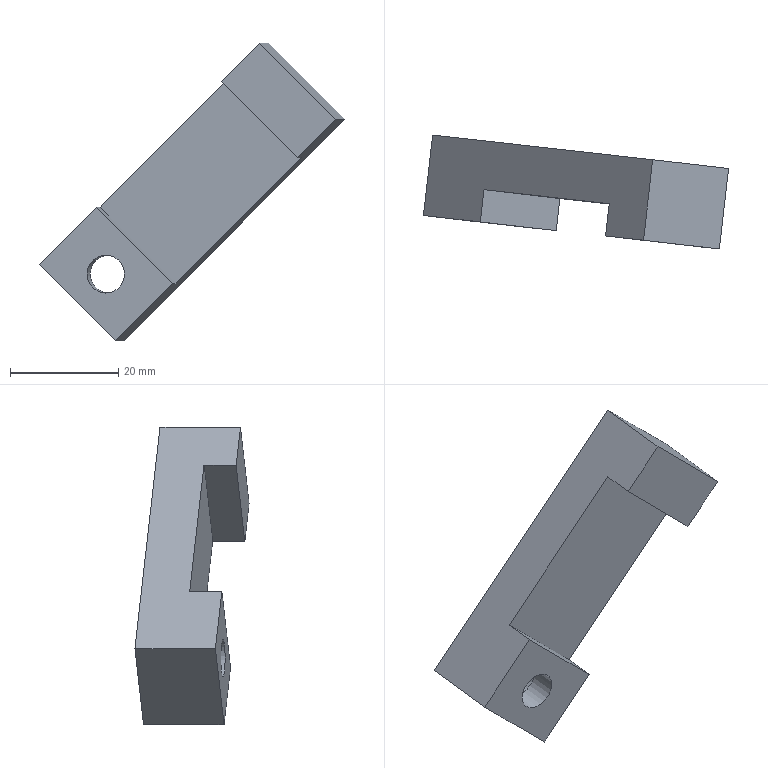Part | NX | features XQ 2 | 1 solid | 13 faces | box 56.498 x 21.147 x 55.154 mm | volume 12297 mm3 | plane 11 | cylinder 2 | commonest cylinder face diameters 7 x1 11 x1
STEP:
#1=CARTESIAN_POINT('',(3335.667,-230.159,-51.019));
#2=VERTEX_POINT('',#1);
#3=CARTESIAN_POINT('',(3312.483,-227.518,-74.354));
#4=VERTEX_POINT('',#3);
#5=CARTESIAN_POINT('',(3328.642,-229.359,-58.09));
#6=DIRECTION('',(-0.7026,0.08005,-0.7071));
#7=VECTOR('',#6,1000.);
#8=LINE('',#5,#7);
#9=EDGE_CURVE('',#2,#4,#8,.T.);
#10=ORIENTED_EDGE('',*,*,#9,.F.);
#11=CARTESIAN_POINT('',(3321.616,-228.559,-36.877));
#12=VERTEX_POINT('',#11);
#13=CARTESIAN_POINT('',(3328.642,-229.359,-43.948));
#14=DIRECTION('',(-0.7026,0.08005,0.7071));
#15=VECTOR('',#14,1000.);
#16=LINE('',#13,#15);
#17=EDGE_CURVE('',#2,#12,#16,.T.);
#18=ORIENTED_EDGE('',*,*,#17,.T.);
#19=CARTESIAN_POINT('',(3298.432,-225.917,-60.211));
#20=VERTEX_POINT('',#19);
#21=CARTESIAN_POINT('',(3314.591,-227.758,-43.948));
#22=DIRECTION('',(0.7026,-0.08005,0.7071));
#23=VECTOR('',#22,1000.);
#24=LINE('',#21,#23);
#25=EDGE_CURVE('',#20,#12,#24,.T.);
#26=ORIENTED_EDGE('',*,*,#25,.F.);
#27=CARTESIAN_POINT('',(3305.457,-226.717,-67.283));
#28=DIRECTION('',(0.7026,-0.08005,-0.7071));
#29=VECTOR('',#28,1000.);
#30=LINE('',#27,#29);
#31=EDGE_CURVE('',#20,#4,#30,.T.);
#32=ORIENTED_EDGE('',*,*,#31,.T.);
#33=EDGE_LOOP('',(#10,#18,#26,#32));
#34=FACE_BOUND('',#33,.T.);
#35=CARTESIAN_POINT('',(3330.93,-229.62,-30.244));
#36=DIRECTION('',(-0.1132,-0.9936,-0.000000218));
#37=DIRECTION('',(-0.000000567,0.000000284,-1.));
#38=AXIS2_PLACEMENT_3D('',#35,#36,#37);
#39=PLANE('',#38);
#40=ADVANCED_FACE('',(#34),#39,.T.);
#41=CARTESIAN_POINT('',(3288.912,-215.774,-70.818));
#42=VERTEX_POINT('',#41);
#43=CARTESIAN_POINT('',(3287.214,-230.678,-70.818));
#44=VERTEX_POINT('',#43);
#45=CARTESIAN_POINT('',(3287.78,-225.71,-70.818));
#46=DIRECTION('',(-0.1132,-0.9936,-0.000000275));
#47=VECTOR('',#46,1000.);
#48=LINE('',#45,#47);
#49=EDGE_CURVE('',#42,#44,#48,.T.);
#50=ORIENTED_EDGE('',*,*,#49,.F.);
#51=CARTESIAN_POINT('',(3302.963,-217.375,-84.96));
#52=VERTEX_POINT('',#51);
#53=CARTESIAN_POINT('',(3297.694,-216.775,-79.657));
#54=DIRECTION('',(-0.7026,0.08005,0.7071));
#55=VECTOR('',#54,1000.);
#56=LINE('',#53,#55);
#57=EDGE_CURVE('',#52,#42,#56,.T.);
#58=ORIENTED_EDGE('',*,*,#57,.F.);
#59=CARTESIAN_POINT('',(3301.265,-232.279,-84.96));
#60=VERTEX_POINT('',#59);
#61=CARTESIAN_POINT('',(3301.831,-227.311,-84.96));
#62=DIRECTION('',(0.1132,0.9936,0.000000275));
#63=VECTOR('',#62,1000.);
#64=LINE('',#61,#63);
#65=EDGE_CURVE('',#60,#52,#64,.T.);
#66=ORIENTED_EDGE('',*,*,#65,.F.);
#67=CARTESIAN_POINT('',(3295.996,-231.678,-79.657));
#68=DIRECTION('',(0.7026,-0.08005,-0.7071));
#69=VECTOR('',#68,1000.);
#70=LINE('',#67,#69);
#71=EDGE_CURVE('',#44,#60,#70,.T.);
#72=ORIENTED_EDGE('',*,*,#71,.F.);
#73=EDGE_LOOP('',(#50,#58,#66,#72));
#74=FACE_BOUND('',#73,.T.);
#75=CARTESIAN_POINT('',(3296.562,-226.71,-79.657));
#76=DIRECTION('',(-0.7026,0.08005,-0.7071));
#77=DIRECTION('',(0.6832,-0.2024,-0.7017));
#78=AXIS2_PLACEMENT_3D('',#75,#76,#77);
#79=PLANE('',#78);
#80=ADVANCED_FACE('',(#74),#79,.T.);
#81=ORIENTED_EDGE('',*,*,#25,.T.);
#82=CARTESIAN_POINT('',(3320.937,-234.52,-36.877));
#83=VERTEX_POINT('',#82);
#84=CARTESIAN_POINT('',(3321.503,-229.552,-36.877));
#85=DIRECTION('',(0.1132,0.9936,0.000000275));
#86=VECTOR('',#85,1000.);
#87=LINE('',#84,#86);
#88=EDGE_CURVE('',#83,#12,#87,.T.);
#89=ORIENTED_EDGE('',*,*,#88,.F.);
#90=CARTESIAN_POINT('',(3327.963,-235.32,-29.806));
#91=VERTEX_POINT('',#90);
#92=CARTESIAN_POINT('',(3313.911,-233.72,-43.948));
#93=DIRECTION('',(0.7026,-0.08005,0.7071));
#94=VECTOR('',#93,1000.);
#95=LINE('',#92,#94);
#96=EDGE_CURVE('',#83,#91,#95,.T.);
#97=ORIENTED_EDGE('',*,*,#96,.T.);
#98=CARTESIAN_POINT('',(3329.661,-220.417,-29.806));
#99=VERTEX_POINT('',#98);
#100=CARTESIAN_POINT('',(3328.529,-230.353,-29.806));
#101=DIRECTION('',(0.1132,0.9936,0.000000275));
#102=VECTOR('',#101,1000.);
#103=LINE('',#100,#102);
#104=EDGE_CURVE('',#91,#99,#103,.T.);
#105=ORIENTED_EDGE('',*,*,#104,.T.);
#106=CARTESIAN_POINT('',(3315.609,-218.816,-43.948));
#107=DIRECTION('',(0.7026,-0.08005,0.7071));
#108=VECTOR('',#107,1000.);
#109=LINE('',#106,#108);
#110=EDGE_CURVE('',#42,#99,#109,.T.);
#111=ORIENTED_EDGE('',*,*,#110,.F.);
#112=ORIENTED_EDGE('',*,*,#49,.T.);
#113=CARTESIAN_POINT('',(3297.752,-231.878,-60.211));
#114=VERTEX_POINT('',#113);
#115=CARTESIAN_POINT('',(3313.911,-233.72,-43.948));
#116=DIRECTION('',(0.7026,-0.08005,0.7071));
#117=VECTOR('',#116,1000.);
#118=LINE('',#115,#117);
#119=EDGE_CURVE('',#44,#114,#118,.T.);
#120=ORIENTED_EDGE('',*,*,#119,.T.);
#121=CARTESIAN_POINT('',(3298.318,-226.911,-60.211));
#122=DIRECTION('',(0.1132,0.9936,0.000000275));
#123=VECTOR('',#122,1000.);
#124=LINE('',#121,#123);
#125=EDGE_CURVE('',#114,#20,#124,.T.);
#126=ORIENTED_EDGE('',*,*,#125,.T.);
#127=EDGE_LOOP('',(#81,#89,#97,#105,#111,#112,#120,#126));
#128=FACE_BOUND('',#127,.T.);
#129=CARTESIAN_POINT('',(3314.477,-228.752,-43.948));
#130=DIRECTION('',(-0.7026,0.08005,0.7071));
#131=DIRECTION('',(-0.7112,-0.0435,-0.7017));
#132=AXIS2_PLACEMENT_3D('',#129,#130,#131);
#133=PLANE('',#132);
#134=ADVANCED_FACE('',(#128),#133,.T.);
#135=ORIENTED_EDGE('',*,*,#9,.T.);
#136=CARTESIAN_POINT('',(3311.804,-233.479,-74.354));
#137=VERTEX_POINT('',#136);
#138=CARTESIAN_POINT('',(3312.37,-228.511,-74.354));
#139=DIRECTION('',(0.1132,0.9936,0.000000275));
#140=VECTOR('',#139,1000.);
#141=LINE('',#138,#140);
#142=EDGE_CURVE('',#137,#4,#141,.T.);
#143=ORIENTED_EDGE('',*,*,#142,.F.);
#144=CARTESIAN_POINT('',(3327.963,-235.32,-58.09));
#145=DIRECTION('',(0.7026,-0.08005,0.7071));
#146=VECTOR('',#145,1000.);
#147=LINE('',#144,#146);
#148=EDGE_CURVE('',#60,#137,#147,.T.);
#149=ORIENTED_EDGE('',*,*,#148,.F.);
#150=ORIENTED_EDGE('',*,*,#65,.T.);
#151=CARTESIAN_POINT('',(3343.712,-222.018,-43.948));
#152=VERTEX_POINT('',#151);
#153=CARTESIAN_POINT('',(3329.661,-220.417,-58.09));
#154=DIRECTION('',(0.7026,-0.08005,0.7071));
#155=VECTOR('',#154,1000.);
#156=LINE('',#153,#155);
#157=EDGE_CURVE('',#52,#152,#156,.T.);
#158=ORIENTED_EDGE('',*,*,#157,.T.);
#159=CARTESIAN_POINT('',(3342.014,-236.921,-43.948));
#160=VERTEX_POINT('',#159);
#161=CARTESIAN_POINT('',(3342.58,-231.954,-43.948));
#162=DIRECTION('',(-0.1132,-0.9936,-0.000000275));
#163=VECTOR('',#162,1000.);
#164=LINE('',#161,#163);
#165=EDGE_CURVE('',#152,#160,#164,.T.);
#166=ORIENTED_EDGE('',*,*,#165,.T.);
#167=CARTESIAN_POINT('',(3334.988,-236.121,-51.019));
#168=VERTEX_POINT('',#167);
#169=CARTESIAN_POINT('',(3327.963,-235.32,-58.09));
#170=DIRECTION('',(0.7026,-0.08005,0.7071));
#171=VECTOR('',#170,1000.);
#172=LINE('',#169,#171);
#173=EDGE_CURVE('',#168,#160,#172,.T.);
#174=ORIENTED_EDGE('',*,*,#173,.F.);
#175=CARTESIAN_POINT('',(3335.554,-231.153,-51.019));
#176=DIRECTION('',(0.1132,0.9936,0.000000275));
#177=VECTOR('',#176,1000.);
#178=LINE('',#175,#177);
#179=EDGE_CURVE('',#168,#2,#178,.T.);
#180=ORIENTED_EDGE('',*,*,#179,.T.);
#181=EDGE_LOOP('',(#135,#143,#149,#150,#158,#166,#174,#180));
#182=FACE_BOUND('',#181,.T.);
#183=CARTESIAN_POINT('',(3328.529,-230.353,-58.09));
#184=DIRECTION('',(0.7026,-0.08005,-0.7071));
#185=DIRECTION('',(0.7112,0.0435,0.7017));
#186=AXIS2_PLACEMENT_3D('',#183,#184,#185);
#187=PLANE('',#186);
#188=ADVANCED_FACE('',(#182),#187,.T.);
#189=ORIENTED_EDGE('',*,*,#165,.F.);
#190=CARTESIAN_POINT('',(3338.443,-221.417,-38.645));
#191=DIRECTION('',(0.7026,-0.08005,-0.7071));
#192=VECTOR('',#191,1000.);
#193=LINE('',#190,#192);
#194=EDGE_CURVE('',#99,#152,#193,.T.);
#195=ORIENTED_EDGE('',*,*,#194,.F.);
#196=ORIENTED_EDGE('',*,*,#104,.F.);
#197=CARTESIAN_POINT('',(3336.745,-236.321,-38.645));
#198=DIRECTION('',(-0.7026,0.08005,0.7071));
#199=VECTOR('',#198,1000.);
#200=LINE('',#197,#199);
#201=EDGE_CURVE('',#160,#91,#200,.T.);
#202=ORIENTED_EDGE('',*,*,#201,.F.);
#203=EDGE_LOOP('',(#189,#195,#196,#202));
#204=FACE_BOUND('',#203,.T.);
#205=CARTESIAN_POINT('',(3337.311,-231.353,-38.645));
#206=DIRECTION('',(0.7026,-0.08005,0.7071));
#207=DIRECTION('',(-0.6832,0.2024,0.7017));
#208=AXIS2_PLACEMENT_3D('',#205,#206,#207);
#209=PLANE('',#208);
#210=ADVANCED_FACE('',(#204),#209,.T.);
#211=ORIENTED_EDGE('',*,*,#110,.T.);
#212=ORIENTED_EDGE('',*,*,#194,.T.);
#213=ORIENTED_EDGE('',*,*,#157,.F.);
#214=ORIENTED_EDGE('',*,*,#57,.T.);
#215=EDGE_LOOP('',(#211,#212,#213,#214));
#216=FACE_BOUND('',#215,.T.);
#217=CARTESIAN_POINT('',(3306.672,-217.798,-72.586));
#218=VERTEX_POINT('',#217);
#219=CARTESIAN_POINT('',(3301.207,-217.175,-72.586));
#220=DIRECTION('',(-0.1132,-0.9936,-0.000000275));
#221=DIRECTION('',(0.9936,-0.1132,0.));
#222=AXIS2_PLACEMENT_3D('',#219,#220,#221);
#223=CIRCLE('',#222,5.5);
#224=EDGE_CURVE('',#218,#218,#223,.T.);
#225=ORIENTED_EDGE('',*,*,#224,.T.);
#226=EDGE_LOOP('',(#225));
#227=FACE_BOUND('',#226,.T.);
#228=CARTESIAN_POINT('',(3324.391,-219.817,-52.787));
#229=DIRECTION('',(0.1132,0.9936,0.000000275));
#230=DIRECTION('',(0.000000561,-0.000000341,1.));
#231=AXIS2_PLACEMENT_3D('',#228,#229,#230);
#232=PLANE('',#231);
#233=ADVANCED_FACE('',(#216,#227),#232,.T.);
#234=CARTESIAN_POINT('',(3305.54,-227.733,-72.586));
#235=VERTEX_POINT('',#234);
#236=CARTESIAN_POINT('',(3300.075,-227.111,-72.586));
#237=DIRECTION('',(-0.1132,-0.9936,-0.000000275));
#238=DIRECTION('',(0.9936,-0.1132,0.));
#239=AXIS2_PLACEMENT_3D('',#236,#237,#238);
#240=CIRCLE('',#239,5.5);
#241=EDGE_CURVE('',#235,#235,#240,.T.);
#242=ORIENTED_EDGE('',*,*,#241,.T.);
#243=EDGE_LOOP('',(#242));
#244=FACE_BOUND('',#243,.T.);
#245=ORIENTED_EDGE('',*,*,#224,.F.);
#246=EDGE_LOOP('',(#245));
#247=FACE_BOUND('',#246,.T.);
#248=CARTESIAN_POINT('',(3300.641,-222.143,-72.586));
#249=DIRECTION('',(-0.1132,-0.9936,-0.000000275));
#250=DIRECTION('',(0.1725,-0.01966,-0.9848));
#251=AXIS2_PLACEMENT_3D('',#248,#249,#250);
#252=CYLINDRICAL_SURFACE('',#251,5.5);
#253=ADVANCED_FACE('',(#244,#247),#252,.F.);
#254=CARTESIAN_POINT('',(3300.075,-227.111,-69.086));
#255=VERTEX_POINT('',#254);
#256=CARTESIAN_POINT('',(3300.075,-227.111,-72.586));
#257=DIRECTION('',(0.1132,0.9936,0.000000275));
#258=DIRECTION('',(0.000000561,-0.000000341,1.));
#259=AXIS2_PLACEMENT_3D('',#256,#257,#258);
#260=CIRCLE('',#259,3.5);
#261=EDGE_CURVE('',#255,#255,#260,.T.);
#262=ORIENTED_EDGE('',*,*,#261,.F.);
#263=EDGE_LOOP('',(#262));
#264=FACE_BOUND('',#263,.T.);
#265=ORIENTED_EDGE('',*,*,#241,.F.);
#266=EDGE_LOOP('',(#265));
#267=FACE_BOUND('',#266,.T.);
#268=CARTESIAN_POINT('',(3300.075,-227.111,-72.586));
#269=DIRECTION('',(0.1132,0.9936,0.000000275));
#270=DIRECTION('',(0.000000561,-0.000000341,1.));
#271=AXIS2_PLACEMENT_3D('',#268,#269,#270);
#272=PLANE('',#271);
#273=ADVANCED_FACE('',(#264,#267),#272,.T.);
#274=ORIENTED_EDGE('',*,*,#31,.F.);
#275=ORIENTED_EDGE('',*,*,#125,.F.);
#276=CARTESIAN_POINT('',(3306.534,-232.879,-69.05));
#277=DIRECTION('',(0.7026,-0.08005,-0.7071));
#278=VECTOR('',#277,1000.);
#279=LINE('',#276,#278);
#280=EDGE_CURVE('',#114,#137,#279,.T.);
#281=ORIENTED_EDGE('',*,*,#280,.T.);
#282=ORIENTED_EDGE('',*,*,#142,.T.);
#283=EDGE_LOOP('',(#274,#275,#281,#282));
#284=FACE_BOUND('',#283,.T.);
#285=CARTESIAN_POINT('',(3305.344,-227.711,-67.283));
#286=DIRECTION('',(0.7026,-0.08005,0.7071));
#287=DIRECTION('',(-0.6832,0.2024,0.7017));
#288=AXIS2_PLACEMENT_3D('',#285,#286,#287);
#289=PLANE('',#288);
#290=ADVANCED_FACE('',(#284),#289,.T.);
#291=CARTESIAN_POINT('',(3299.509,-232.079,-76.086));
#292=VERTEX_POINT('',#291);
#293=CARTESIAN_POINT('',(3299.509,-232.079,-72.586));
#294=DIRECTION('',(-0.1132,-0.9936,-0.000000275));
#295=DIRECTION('',(-0.000000561,0.000000341,-1.));
#296=AXIS2_PLACEMENT_3D('',#293,#294,#295);
#297=CIRCLE('',#296,3.5);
#298=EDGE_CURVE('',#292,#292,#297,.T.);
#299=ORIENTED_EDGE('',*,*,#298,.F.);
#300=EDGE_LOOP('',(#299));
#301=FACE_BOUND('',#300,.T.);
#302=ORIENTED_EDGE('',*,*,#119,.F.);
#303=ORIENTED_EDGE('',*,*,#71,.T.);
#304=ORIENTED_EDGE('',*,*,#148,.T.);
#305=ORIENTED_EDGE('',*,*,#280,.F.);
#306=EDGE_LOOP('',(#302,#303,#304,#305));
#307=FACE_BOUND('',#306,.T.);
#308=CARTESIAN_POINT('',(3322.693,-234.72,-52.787));
#309=DIRECTION('',(-0.1132,-0.9936,-0.000000275));
#310=DIRECTION('',(-0.000000561,0.000000341,-1.));
#311=AXIS2_PLACEMENT_3D('',#308,#309,#310);
#312=PLANE('',#311);
#313=ADVANCED_FACE('',(#301,#307),#312,.T.);
#314=ORIENTED_EDGE('',*,*,#298,.T.);
#315=EDGE_LOOP('',(#314));
#316=FACE_BOUND('',#315,.T.);
#317=ORIENTED_EDGE('',*,*,#261,.T.);
#318=EDGE_LOOP('',(#317));
#319=FACE_BOUND('',#318,.T.);
#320=CARTESIAN_POINT('',(3300.641,-222.143,-72.586));
#321=DIRECTION('',(-0.1132,-0.9936,-0.000000275));
#322=DIRECTION('',(0.1725,-0.01966,-0.9848));
#323=AXIS2_PLACEMENT_3D('',#320,#321,#322);
#324=CYLINDRICAL_SURFACE('',#323,3.5);
#325=ADVANCED_FACE('',(#316,#319),#324,.F.);
#326=ORIENTED_EDGE('',*,*,#17,.F.);
#327=ORIENTED_EDGE('',*,*,#179,.F.);
#328=CARTESIAN_POINT('',(3329.719,-235.521,-45.716));
#329=DIRECTION('',(0.7026,-0.08005,-0.7071));
#330=VECTOR('',#329,1000.);
#331=LINE('',#328,#330);
#332=EDGE_CURVE('',#83,#168,#331,.T.);
#333=ORIENTED_EDGE('',*,*,#332,.F.);
#334=ORIENTED_EDGE('',*,*,#88,.T.);
#335=EDGE_LOOP('',(#326,#327,#333,#334));
#336=FACE_BOUND('',#335,.T.);
#337=CARTESIAN_POINT('',(3328.529,-230.353,-43.948));
#338=DIRECTION('',(-0.7026,0.08005,-0.7071));
#339=DIRECTION('',(0.6832,-0.2024,-0.7017));
#340=AXIS2_PLACEMENT_3D('',#337,#338,#339);
#341=PLANE('',#340);
#342=ADVANCED_FACE('',(#336),#341,.T.);
#343=ORIENTED_EDGE('',*,*,#173,.T.);
#344=ORIENTED_EDGE('',*,*,#201,.T.);
#345=ORIENTED_EDGE('',*,*,#96,.F.);
#346=ORIENTED_EDGE('',*,*,#332,.T.);
#347=EDGE_LOOP('',(#343,#344,#345,#346));
#348=FACE_BOUND('',#347,.T.);
#349=CARTESIAN_POINT('',(3322.693,-234.72,-52.787));
#350=DIRECTION('',(-0.1132,-0.9936,-0.000000275));
#351=DIRECTION('',(-0.000000561,0.000000341,-1.));
#352=AXIS2_PLACEMENT_3D('',#349,#350,#351);
#353=PLANE('',#352);
#354=ADVANCED_FACE('',(#348),#353,.T.);
#355=CLOSED_SHELL('',(#40,#80,#134,#188,#210,#233,#253,#273,#290,#313,#325,#342,#354));
#356=MANIFOLD_SOLID_BREP('',#355);
#357=(LENGTH_UNIT()NAMED_UNIT(*)SI_UNIT(.MILLI.,.METRE.));
#358=UNCERTAINTY_MEASURE_WITH_UNIT(LENGTH_MEASURE(0.00001),#357,'','');
#359=(NAMED_UNIT(*)PLANE_ANGLE_UNIT()SI_UNIT($,.RADIAN.));
#360=(NAMED_UNIT(*)SI_UNIT($,.STERADIAN.)SOLID_ANGLE_UNIT());
#361=(GEOMETRIC_REPRESENTATION_CONTEXT(3)GLOBAL_UNCERTAINTY_ASSIGNED_CONTEXT((#358))GLOBAL_UNIT_ASSIGNED_CONTEXT((#357,#359,#360))REPRESENTATION_CONTEXT('',''));
#362=ADVANCED_BREP_SHAPE_REPRESENTATION('',(#356),#361);